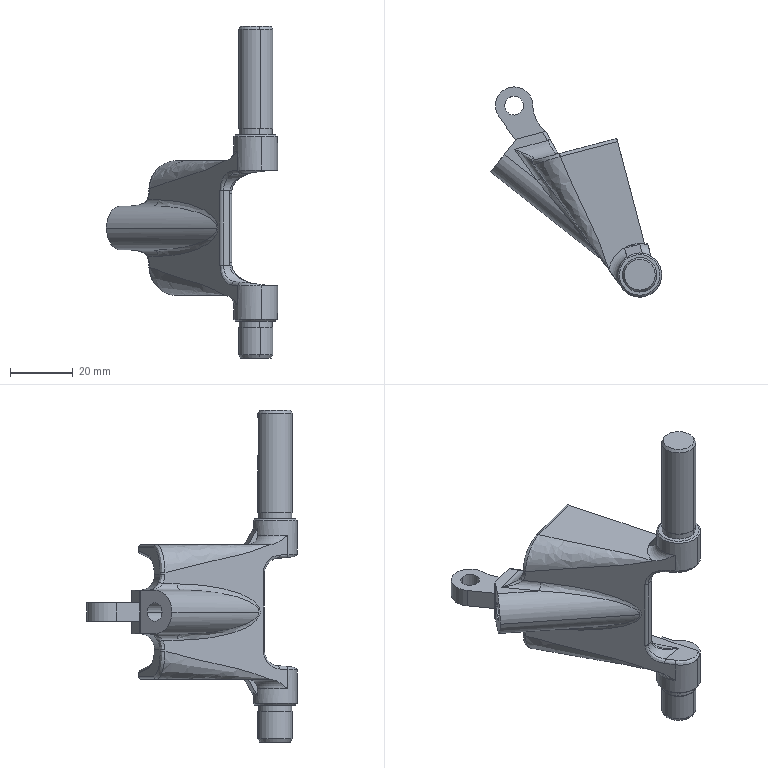Part | SolidWorks | features BaseBody 1 | 1 solid | 128 faces | box 54.652 x 67.08 x 106 mm | volume 26599 mm3 | cylinder 47 | plane 45 | spline 24 | cone 8 | torus 4 | commonest cylinder face diameters 2 x15 14 x8 6 x4 10 x4 10.6 x4 11 x4